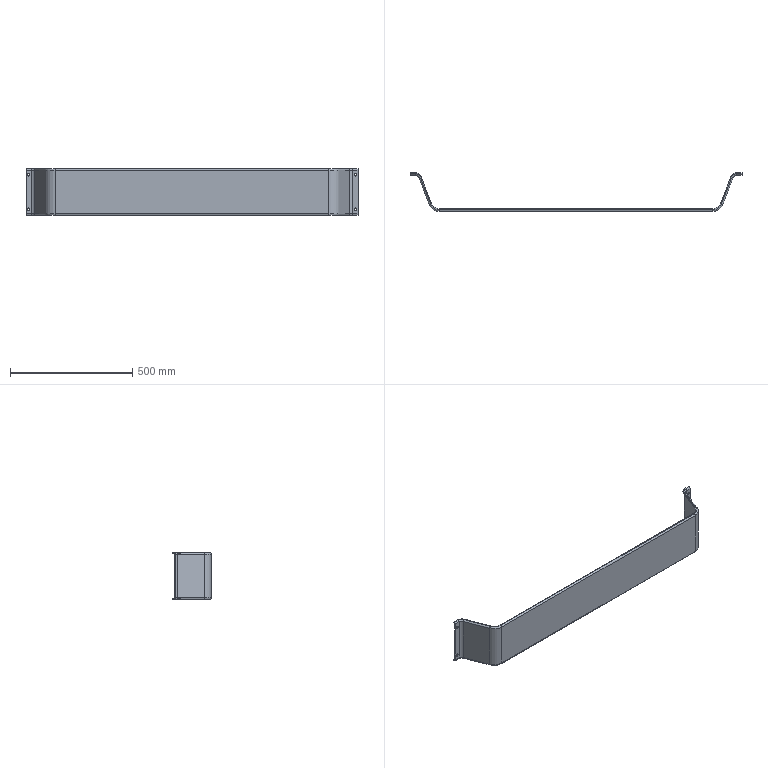Part | SolidWorks | features Fillet 8, ICE 7, Extrusion 1, HoleWzd 1 | 1 solid | 86 faces | box 1359 x 158.842 x 192 mm | volume 1237000 mm3 | cylinder 44 | plane 26 | torus 16 | commonest cylinder face diameters 4 x10 12 x10 10 x8 52 x4 68 x4 32 x2